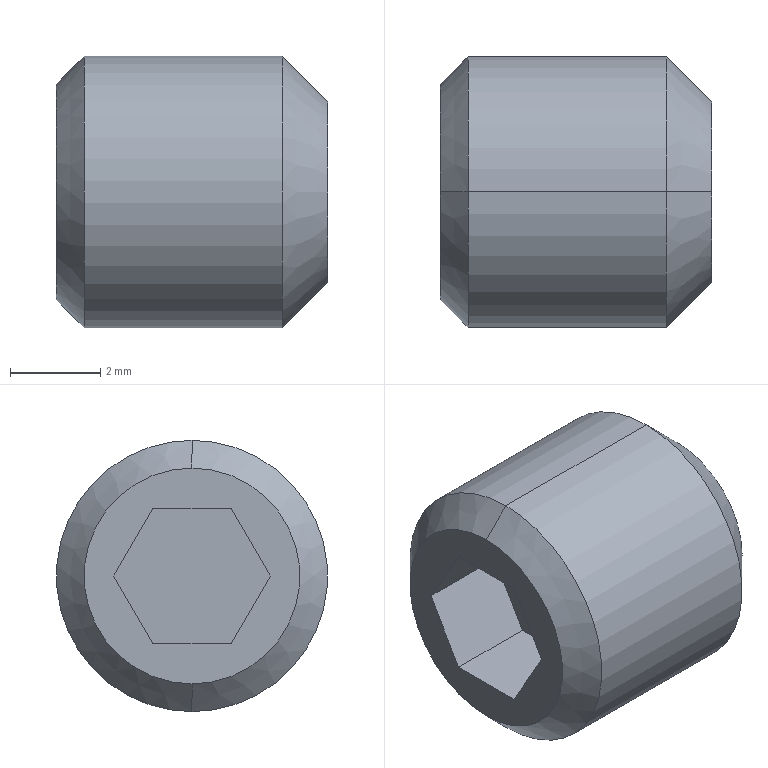Part | STEP file | MSSFS6-6-4 | 1 solid | 15 faces | box 6 x 6 x 6 mm | volume 142.374 mm3 | plane 9 | cone 4 | cylinder 2 | commonest cylinder face diameters 6 x2
STEP:
#1=CARTESIAN_POINT('',(0.,0.,2.387));
#2=VERTEX_POINT('',#1);
#3=CARTESIAN_POINT('',(0.,0.,-2.387));
#4=VERTEX_POINT('',#3);
#5=CARTESIAN_POINT('',(0.,0.,0.));
#6=DIRECTION('',(-1.,0.,0.));
#7=DIRECTION('',(0.,0.,1.));
#8=AXIS2_PLACEMENT_3D('',#5,#6,#7);
#9=CIRCLE('',#8,2.387);
#10=EDGE_CURVE('',#2,#4,#9,.T.);
#11=ORIENTED_EDGE('',*,*,#10,.F.);
#12=CARTESIAN_POINT('',(0.6135,0.,3.));
#13=VERTEX_POINT('',#12);
#14=CARTESIAN_POINT('',(0.,0.,2.387));
#15=DIRECTION('',(0.7071,0.,0.7071));
#16=VECTOR('',#15,1000.);
#17=LINE('',#14,#16);
#18=EDGE_CURVE('',#2,#13,#17,.T.);
#19=ORIENTED_EDGE('',*,*,#18,.T.);
#20=CARTESIAN_POINT('',(0.6135,0.,-3.));
#21=VERTEX_POINT('',#20);
#22=CARTESIAN_POINT('',(0.6135,0.,0.));
#23=DIRECTION('',(-1.,0.,0.));
#24=DIRECTION('',(0.,0.,1.));
#25=AXIS2_PLACEMENT_3D('',#22,#23,#24);
#26=CIRCLE('',#25,3.);
#27=EDGE_CURVE('',#13,#21,#26,.T.);
#28=ORIENTED_EDGE('',*,*,#27,.T.);
#29=CARTESIAN_POINT('',(0.,0.,-2.387));
#30=DIRECTION('',(0.7071,0.,-0.7071));
#31=VECTOR('',#30,1000.);
#32=LINE('',#29,#31);
#33=EDGE_CURVE('',#4,#21,#32,.T.);
#34=ORIENTED_EDGE('',*,*,#33,.F.);
#35=EDGE_LOOP('',(#11,#19,#28,#34));
#36=FACE_OUTER_BOUND('',#35,.T.);
#37=CARTESIAN_POINT('',(0.,0.,0.));
#38=DIRECTION('',(1.,0.,0.));
#39=DIRECTION('',(0.,0.,-1.));
#40=AXIS2_PLACEMENT_3D('',#37,#38,#39);
#41=CONICAL_SURFACE('',#40,2.387,0.7854);
#42=ADVANCED_FACE('',(#36),#41,.T.);
#43=CARTESIAN_POINT('',(5.,0.,3.));
#44=VERTEX_POINT('',#43);
#45=CARTESIAN_POINT('',(5.,0.,-3.));
#46=VERTEX_POINT('',#45);
#47=CARTESIAN_POINT('',(5.,0.,0.));
#48=DIRECTION('',(-1.,0.,0.));
#49=DIRECTION('',(0.,0.,1.));
#50=AXIS2_PLACEMENT_3D('',#47,#48,#49);
#51=CIRCLE('',#50,3.);
#52=EDGE_CURVE('',#44,#46,#51,.T.);
#53=ORIENTED_EDGE('',*,*,#52,.T.);
#54=CARTESIAN_POINT('',(-1.,0.,-3.));
#55=DIRECTION('',(-1.,0.,0.));
#56=VECTOR('',#55,1000.);
#57=LINE('',#54,#56);
#58=EDGE_CURVE('',#46,#21,#57,.T.);
#59=ORIENTED_EDGE('',*,*,#58,.T.);
#60=ORIENTED_EDGE('',*,*,#27,.F.);
#61=CARTESIAN_POINT('',(-1.,0.,3.));
#62=DIRECTION('',(-1.,0.,0.));
#63=VECTOR('',#62,1000.);
#64=LINE('',#61,#63);
#65=EDGE_CURVE('',#44,#13,#64,.T.);
#66=ORIENTED_EDGE('',*,*,#65,.F.);
#67=EDGE_LOOP('',(#53,#59,#60,#66));
#68=FACE_OUTER_BOUND('',#67,.T.);
#69=CARTESIAN_POINT('',(-1.,0.,0.));
#70=DIRECTION('',(-1.,0.,0.));
#71=DIRECTION('',(0.,0.,1.));
#72=AXIS2_PLACEMENT_3D('',#69,#70,#71);
#73=CYLINDRICAL_SURFACE('',#72,3.);
#74=ADVANCED_FACE('',(#68),#73,.T.);
#75=CARTESIAN_POINT('',(6.,0.,2.));
#76=VERTEX_POINT('',#75);
#77=CARTESIAN_POINT('',(6.,0.,-2.));
#78=VERTEX_POINT('',#77);
#79=CARTESIAN_POINT('',(6.,0.,0.));
#80=DIRECTION('',(-1.,0.,0.));
#81=DIRECTION('',(0.,0.,1.));
#82=AXIS2_PLACEMENT_3D('',#79,#80,#81);
#83=CIRCLE('',#82,2.);
#84=EDGE_CURVE('',#76,#78,#83,.T.);
#85=ORIENTED_EDGE('',*,*,#84,.T.);
#86=CARTESIAN_POINT('',(5.,0.,-3.));
#87=DIRECTION('',(-0.7071,0.,-0.7071));
#88=VECTOR('',#87,1000.);
#89=LINE('',#86,#88);
#90=EDGE_CURVE('',#78,#46,#89,.T.);
#91=ORIENTED_EDGE('',*,*,#90,.T.);
#92=ORIENTED_EDGE('',*,*,#52,.F.);
#93=CARTESIAN_POINT('',(5.,0.,3.));
#94=DIRECTION('',(-0.7071,0.,0.7071));
#95=VECTOR('',#94,1000.);
#96=LINE('',#93,#95);
#97=EDGE_CURVE('',#76,#44,#96,.T.);
#98=ORIENTED_EDGE('',*,*,#97,.F.);
#99=EDGE_LOOP('',(#85,#91,#92,#98));
#100=FACE_OUTER_BOUND('',#99,.T.);
#101=CARTESIAN_POINT('',(5.,0.,0.));
#102=DIRECTION('',(-1.,0.,0.));
#103=DIRECTION('',(0.,0.,1.));
#104=AXIS2_PLACEMENT_3D('',#101,#102,#103);
#105=CONICAL_SURFACE('',#104,3.,0.7854);
#106=ADVANCED_FACE('',(#100),#105,.T.);
#107=CARTESIAN_POINT('',(0.,0.866,1.5));
#108=VERTEX_POINT('',#107);
#109=CARTESIAN_POINT('',(0.,1.732,0.));
#110=VERTEX_POINT('',#109);
#111=CARTESIAN_POINT('',(0.,0.866,1.5));
#112=DIRECTION('',(0.,0.5,-0.866));
#113=VECTOR('',#112,1000.);
#114=LINE('',#111,#113);
#115=EDGE_CURVE('',#108,#110,#114,.T.);
#116=ORIENTED_EDGE('',*,*,#115,.F.);
#117=CARTESIAN_POINT('',(0.,-0.866,1.5));
#118=VERTEX_POINT('',#117);
#119=CARTESIAN_POINT('',(0.,-0.866,1.5));
#120=DIRECTION('',(0.,1.,0.));
#121=VECTOR('',#120,1000.);
#122=LINE('',#119,#121);
#123=EDGE_CURVE('',#118,#108,#122,.T.);
#124=ORIENTED_EDGE('',*,*,#123,.F.);
#125=CARTESIAN_POINT('',(0.,-1.732,0.));
#126=VERTEX_POINT('',#125);
#127=CARTESIAN_POINT('',(0.,-1.732,0.));
#128=DIRECTION('',(0.,0.5,0.866));
#129=VECTOR('',#128,1000.);
#130=LINE('',#127,#129);
#131=EDGE_CURVE('',#126,#118,#130,.T.);
#132=ORIENTED_EDGE('',*,*,#131,.F.);
#133=CARTESIAN_POINT('',(0.,-0.866,-1.5));
#134=VERTEX_POINT('',#133);
#135=CARTESIAN_POINT('',(0.,-0.866,-1.5));
#136=DIRECTION('',(0.,-0.5,0.866));
#137=VECTOR('',#136,1000.);
#138=LINE('',#135,#137);
#139=EDGE_CURVE('',#134,#126,#138,.T.);
#140=ORIENTED_EDGE('',*,*,#139,.F.);
#141=CARTESIAN_POINT('',(0.,0.866,-1.5));
#142=VERTEX_POINT('',#141);
#143=CARTESIAN_POINT('',(0.,0.866,-1.5));
#144=DIRECTION('',(0.,-1.,0.));
#145=VECTOR('',#144,1000.);
#146=LINE('',#143,#145);
#147=EDGE_CURVE('',#142,#134,#146,.T.);
#148=ORIENTED_EDGE('',*,*,#147,.F.);
#149=CARTESIAN_POINT('',(0.,1.732,0.));
#150=DIRECTION('',(0.,-0.5,-0.866));
#151=VECTOR('',#150,1000.);
#152=LINE('',#149,#151);
#153=EDGE_CURVE('',#110,#142,#152,.T.);
#154=ORIENTED_EDGE('',*,*,#153,.F.);
#155=EDGE_LOOP('',(#116,#124,#132,#140,#148,#154));
#156=FACE_BOUND('',#155,.T.);
#157=CARTESIAN_POINT('',(0.,0.,0.));
#158=DIRECTION('',(-1.,0.,0.));
#159=DIRECTION('',(0.,0.,1.));
#160=AXIS2_PLACEMENT_3D('',#157,#158,#159);
#161=CIRCLE('',#160,2.387);
#162=EDGE_CURVE('',#4,#2,#161,.T.);
#163=ORIENTED_EDGE('',*,*,#162,.T.);
#164=ORIENTED_EDGE('',*,*,#10,.T.);
#165=EDGE_LOOP('',(#163,#164));
#166=FACE_OUTER_BOUND('',#165,.T.);
#167=CARTESIAN_POINT('',(0.,-2.387,0.));
#168=DIRECTION('',(-1.,0.,0.));
#169=DIRECTION('',(0.,0.,1.));
#170=AXIS2_PLACEMENT_3D('',#167,#168,#169);
#171=PLANE('',#170);
#172=ADVANCED_FACE('',(#156,#166),#171,.T.);
#173=ORIENTED_EDGE('',*,*,#84,.F.);
#174=CARTESIAN_POINT('',(6.,0.,0.));
#175=DIRECTION('',(-1.,0.,0.));
#176=DIRECTION('',(0.,0.,1.));
#177=AXIS2_PLACEMENT_3D('',#174,#175,#176);
#178=CIRCLE('',#177,2.);
#179=EDGE_CURVE('',#78,#76,#178,.T.);
#180=ORIENTED_EDGE('',*,*,#179,.F.);
#181=EDGE_LOOP('',(#173,#180));
#182=FACE_OUTER_BOUND('',#181,.T.);
#183=CARTESIAN_POINT('',(6.,0.,0.));
#184=DIRECTION('',(1.,0.,0.));
#185=DIRECTION('',(0.,0.,-1.));
#186=AXIS2_PLACEMENT_3D('',#183,#184,#185);
#187=PLANE('',#186);
#188=ADVANCED_FACE('',(#182),#187,.T.);
#189=ORIENTED_EDGE('',*,*,#90,.F.);
#190=ORIENTED_EDGE('',*,*,#179,.T.);
#191=ORIENTED_EDGE('',*,*,#97,.T.);
#192=CARTESIAN_POINT('',(5.,0.,0.));
#193=DIRECTION('',(-1.,0.,0.));
#194=DIRECTION('',(0.,0.,1.));
#195=AXIS2_PLACEMENT_3D('',#192,#193,#194);
#196=CIRCLE('',#195,3.);
#197=EDGE_CURVE('',#46,#44,#196,.T.);
#198=ORIENTED_EDGE('',*,*,#197,.F.);
#199=EDGE_LOOP('',(#189,#190,#191,#198));
#200=FACE_OUTER_BOUND('',#199,.T.);
#201=CARTESIAN_POINT('',(5.,0.,0.));
#202=DIRECTION('',(-1.,0.,0.));
#203=DIRECTION('',(0.,0.,1.));
#204=AXIS2_PLACEMENT_3D('',#201,#202,#203);
#205=CONICAL_SURFACE('',#204,3.,0.7854);
#206=ADVANCED_FACE('',(#200),#205,.T.);
#207=ORIENTED_EDGE('',*,*,#58,.F.);
#208=ORIENTED_EDGE('',*,*,#197,.T.);
#209=ORIENTED_EDGE('',*,*,#65,.T.);
#210=CARTESIAN_POINT('',(0.6135,0.,0.));
#211=DIRECTION('',(-1.,0.,0.));
#212=DIRECTION('',(0.,0.,1.));
#213=AXIS2_PLACEMENT_3D('',#210,#211,#212);
#214=CIRCLE('',#213,3.);
#215=EDGE_CURVE('',#21,#13,#214,.T.);
#216=ORIENTED_EDGE('',*,*,#215,.F.);
#217=EDGE_LOOP('',(#207,#208,#209,#216));
#218=FACE_OUTER_BOUND('',#217,.T.);
#219=CARTESIAN_POINT('',(-1.,0.,0.));
#220=DIRECTION('',(-1.,0.,0.));
#221=DIRECTION('',(0.,0.,1.));
#222=AXIS2_PLACEMENT_3D('',#219,#220,#221);
#223=CYLINDRICAL_SURFACE('',#222,3.);
#224=ADVANCED_FACE('',(#218),#223,.T.);
#225=ORIENTED_EDGE('',*,*,#18,.F.);
#226=ORIENTED_EDGE('',*,*,#162,.F.);
#227=ORIENTED_EDGE('',*,*,#33,.T.);
#228=ORIENTED_EDGE('',*,*,#215,.T.);
#229=EDGE_LOOP('',(#225,#226,#227,#228));
#230=FACE_OUTER_BOUND('',#229,.T.);
#231=CARTESIAN_POINT('',(0.,0.,0.));
#232=DIRECTION('',(1.,0.,0.));
#233=DIRECTION('',(0.,0.,-1.));
#234=AXIS2_PLACEMENT_3D('',#231,#232,#233);
#235=CONICAL_SURFACE('',#234,2.387,0.7854);
#236=ADVANCED_FACE('',(#230),#235,.T.);
#237=ORIENTED_EDGE('',*,*,#115,.T.);
#238=CARTESIAN_POINT('',(2.,1.732,0.));
#239=VERTEX_POINT('',#238);
#240=CARTESIAN_POINT('',(2.,1.732,0.));
#241=DIRECTION('',(-1.,0.,0.));
#242=VECTOR('',#241,1000.);
#243=LINE('',#240,#242);
#244=EDGE_CURVE('',#239,#110,#243,.T.);
#245=ORIENTED_EDGE('',*,*,#244,.F.);
#246=CARTESIAN_POINT('',(2.,0.866,1.5));
#247=VERTEX_POINT('',#246);
#248=CARTESIAN_POINT('',(2.,0.866,1.5));
#249=DIRECTION('',(0.,0.5,-0.866));
#250=VECTOR('',#249,1000.);
#251=LINE('',#248,#250);
#252=EDGE_CURVE('',#247,#239,#251,.T.);
#253=ORIENTED_EDGE('',*,*,#252,.F.);
#254=CARTESIAN_POINT('',(2.,0.866,1.5));
#255=DIRECTION('',(-1.,0.,0.));
#256=VECTOR('',#255,1000.);
#257=LINE('',#254,#256);
#258=EDGE_CURVE('',#247,#108,#257,.T.);
#259=ORIENTED_EDGE('',*,*,#258,.T.);
#260=EDGE_LOOP('',(#237,#245,#253,#259));
#261=FACE_OUTER_BOUND('',#260,.T.);
#262=CARTESIAN_POINT('',(2.,0.866,1.5));
#263=DIRECTION('',(0.,0.866,0.5));
#264=DIRECTION('',(0.,-0.5,0.866));
#265=AXIS2_PLACEMENT_3D('',#262,#263,#264);
#266=PLANE('',#265);
#267=ADVANCED_FACE('',(#261),#266,.F.);
#268=ORIENTED_EDGE('',*,*,#123,.T.);
#269=ORIENTED_EDGE('',*,*,#258,.F.);
#270=CARTESIAN_POINT('',(2.,-0.866,1.5));
#271=VERTEX_POINT('',#270);
#272=CARTESIAN_POINT('',(2.,-0.866,1.5));
#273=DIRECTION('',(0.,1.,0.));
#274=VECTOR('',#273,1000.);
#275=LINE('',#272,#274);
#276=EDGE_CURVE('',#271,#247,#275,.T.);
#277=ORIENTED_EDGE('',*,*,#276,.F.);
#278=CARTESIAN_POINT('',(2.,-0.866,1.5));
#279=DIRECTION('',(-1.,0.,0.));
#280=VECTOR('',#279,1000.);
#281=LINE('',#278,#280);
#282=EDGE_CURVE('',#271,#118,#281,.T.);
#283=ORIENTED_EDGE('',*,*,#282,.T.);
#284=EDGE_LOOP('',(#268,#269,#277,#283));
#285=FACE_OUTER_BOUND('',#284,.T.);
#286=CARTESIAN_POINT('',(2.,-0.866,1.5));
#287=DIRECTION('',(0.,0.,1.));
#288=DIRECTION('',(0.,-1.,0.));
#289=AXIS2_PLACEMENT_3D('',#286,#287,#288);
#290=PLANE('',#289);
#291=ADVANCED_FACE('',(#285),#290,.F.);
#292=ORIENTED_EDGE('',*,*,#131,.T.);
#293=ORIENTED_EDGE('',*,*,#282,.F.);
#294=CARTESIAN_POINT('',(2.,-1.732,0.));
#295=VERTEX_POINT('',#294);
#296=CARTESIAN_POINT('',(2.,-1.732,0.));
#297=DIRECTION('',(0.,0.5,0.866));
#298=VECTOR('',#297,1000.);
#299=LINE('',#296,#298);
#300=EDGE_CURVE('',#295,#271,#299,.T.);
#301=ORIENTED_EDGE('',*,*,#300,.F.);
#302=CARTESIAN_POINT('',(2.,-1.732,0.));
#303=DIRECTION('',(-1.,0.,0.));
#304=VECTOR('',#303,1000.);
#305=LINE('',#302,#304);
#306=EDGE_CURVE('',#295,#126,#305,.T.);
#307=ORIENTED_EDGE('',*,*,#306,.T.);
#308=EDGE_LOOP('',(#292,#293,#301,#307));
#309=FACE_OUTER_BOUND('',#308,.T.);
#310=CARTESIAN_POINT('',(2.,-1.732,0.));
#311=DIRECTION('',(0.,-0.866,0.5));
#312=DIRECTION('',(0.,-0.5,-0.866));
#313=AXIS2_PLACEMENT_3D('',#310,#311,#312);
#314=PLANE('',#313);
#315=ADVANCED_FACE('',(#309),#314,.F.);
#316=ORIENTED_EDGE('',*,*,#139,.T.);
#317=ORIENTED_EDGE('',*,*,#306,.F.);
#318=CARTESIAN_POINT('',(2.,-0.866,-1.5));
#319=VERTEX_POINT('',#318);
#320=CARTESIAN_POINT('',(2.,-0.866,-1.5));
#321=DIRECTION('',(0.,-0.5,0.866));
#322=VECTOR('',#321,1000.);
#323=LINE('',#320,#322);
#324=EDGE_CURVE('',#319,#295,#323,.T.);
#325=ORIENTED_EDGE('',*,*,#324,.F.);
#326=CARTESIAN_POINT('',(2.,-0.866,-1.5));
#327=DIRECTION('',(-1.,0.,0.));
#328=VECTOR('',#327,1000.);
#329=LINE('',#326,#328);
#330=EDGE_CURVE('',#319,#134,#329,.T.);
#331=ORIENTED_EDGE('',*,*,#330,.T.);
#332=EDGE_LOOP('',(#316,#317,#325,#331));
#333=FACE_OUTER_BOUND('',#332,.T.);
#334=CARTESIAN_POINT('',(2.,-0.866,-1.5));
#335=DIRECTION('',(0.,-0.866,-0.5));
#336=DIRECTION('',(0.,0.5,-0.866));
#337=AXIS2_PLACEMENT_3D('',#334,#335,#336);
#338=PLANE('',#337);
#339=ADVANCED_FACE('',(#333),#338,.F.);
#340=ORIENTED_EDGE('',*,*,#147,.T.);
#341=ORIENTED_EDGE('',*,*,#330,.F.);
#342=CARTESIAN_POINT('',(2.,0.866,-1.5));
#343=VERTEX_POINT('',#342);
#344=CARTESIAN_POINT('',(2.,0.866,-1.5));
#345=DIRECTION('',(0.,-1.,0.));
#346=VECTOR('',#345,1000.);
#347=LINE('',#344,#346);
#348=EDGE_CURVE('',#343,#319,#347,.T.);
#349=ORIENTED_EDGE('',*,*,#348,.F.);
#350=CARTESIAN_POINT('',(2.,0.866,-1.5));
#351=DIRECTION('',(-1.,0.,0.));
#352=VECTOR('',#351,1000.);
#353=LINE('',#350,#352);
#354=EDGE_CURVE('',#343,#142,#353,.T.);
#355=ORIENTED_EDGE('',*,*,#354,.T.);
#356=EDGE_LOOP('',(#340,#341,#349,#355));
#357=FACE_OUTER_BOUND('',#356,.T.);
#358=CARTESIAN_POINT('',(2.,0.866,-1.5));
#359=DIRECTION('',(0.,0.,-1.));
#360=DIRECTION('',(-1.,0.,0.));
#361=AXIS2_PLACEMENT_3D('',#358,#359,#360);
#362=PLANE('',#361);
#363=ADVANCED_FACE('',(#357),#362,.F.);
#364=ORIENTED_EDGE('',*,*,#153,.T.);
#365=ORIENTED_EDGE('',*,*,#354,.F.);
#366=CARTESIAN_POINT('',(2.,1.732,0.));
#367=DIRECTION('',(0.,-0.5,-0.866));
#368=VECTOR('',#367,1000.);
#369=LINE('',#366,#368);
#370=EDGE_CURVE('',#239,#343,#369,.T.);
#371=ORIENTED_EDGE('',*,*,#370,.F.);
#372=ORIENTED_EDGE('',*,*,#244,.T.);
#373=EDGE_LOOP('',(#364,#365,#371,#372));
#374=FACE_OUTER_BOUND('',#373,.T.);
#375=CARTESIAN_POINT('',(2.,1.732,0.));
#376=DIRECTION('',(0.,0.866,-0.5));
#377=DIRECTION('',(0.,0.5,0.866));
#378=AXIS2_PLACEMENT_3D('',#375,#376,#377);
#379=PLANE('',#378);
#380=ADVANCED_FACE('',(#374),#379,.F.);
#381=ORIENTED_EDGE('',*,*,#252,.T.);
#382=ORIENTED_EDGE('',*,*,#370,.T.);
#383=ORIENTED_EDGE('',*,*,#348,.T.);
#384=ORIENTED_EDGE('',*,*,#324,.T.);
#385=ORIENTED_EDGE('',*,*,#300,.T.);
#386=ORIENTED_EDGE('',*,*,#276,.T.);
#387=EDGE_LOOP('',(#381,#382,#383,#384,#385,#386));
#388=FACE_OUTER_BOUND('',#387,.T.);
#389=CARTESIAN_POINT('',(2.,0.,0.));
#390=DIRECTION('',(-1.,0.,0.));
#391=DIRECTION('',(0.,0.,1.));
#392=AXIS2_PLACEMENT_3D('',#389,#390,#391);
#393=PLANE('',#392);
#394=ADVANCED_FACE('',(#388),#393,.T.);
#395=CLOSED_SHELL('',(#42,#74,#106,#172,#188,#206,#224,#236,#267,#291,#315,#339,#363,#380,#394));
#396=MANIFOLD_SOLID_BREP('',#395);
#397=CARTESIAN_POINT('',(0.,0.,0.));
#398=DIRECTION('',(0.,0.,1.));
#399=DIRECTION('',(1.,0.,0.));
#400=AXIS2_PLACEMENT_3D('',#397,#398,#399);
#401=(LENGTH_UNIT()NAMED_UNIT(*)SI_UNIT(.MILLI.,.METRE.));
#402=UNCERTAINTY_MEASURE_WITH_UNIT(LENGTH_MEASURE(0.00001),#401,'','');
#403=(NAMED_UNIT(*)PLANE_ANGLE_UNIT()SI_UNIT($,.RADIAN.));
#404=(NAMED_UNIT(*)SI_UNIT($,.STERADIAN.)SOLID_ANGLE_UNIT());
#405=(GEOMETRIC_REPRESENTATION_CONTEXT(3)GLOBAL_UNCERTAINTY_ASSIGNED_CONTEXT((#402))GLOBAL_UNIT_ASSIGNED_CONTEXT((#401,#403,#404))REPRESENTATION_CONTEXT('',''));
#406=ADVANCED_BREP_SHAPE_REPRESENTATION('',(#396,#400),#405);